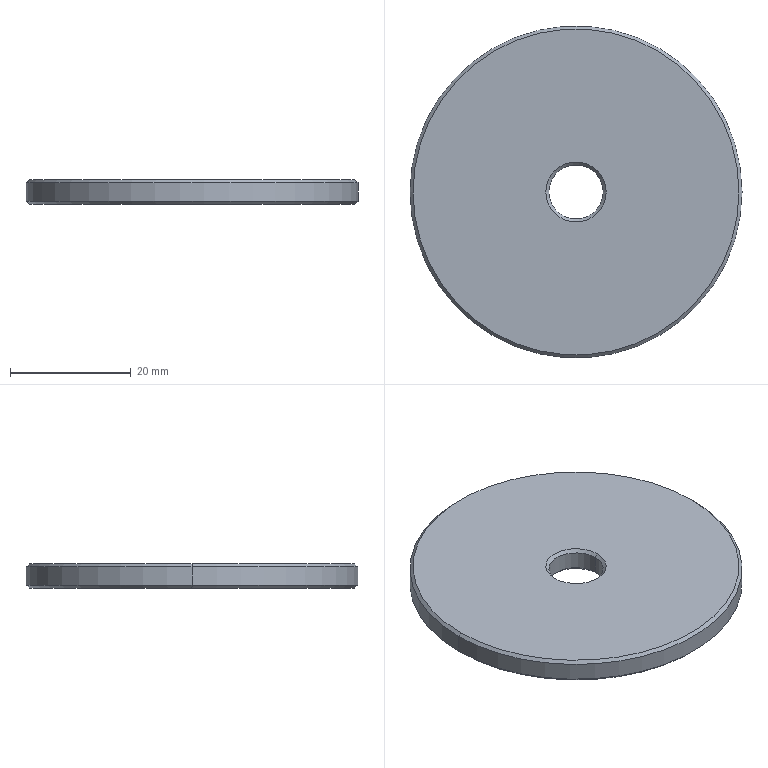Part | SolidWorks | features BaseBody 1 | 1 solid | 14 faces | box 55 x 55 x 4 mm | volume 9199 mm3 | cone 8 | cylinder 4 | plane 2 | commonest cylinder face diameters 9 x2 55 x2
STEP:
#1=CARTESIAN_POINT('',(27.,0.,4.));
#2=VERTEX_POINT('',#1);
#3=CARTESIAN_POINT('',(-27.,0.,4.));
#4=VERTEX_POINT('',#3);
#5=CARTESIAN_POINT('',(0.,0.,4.));
#6=DIRECTION('',(0.,0.,1.));
#7=DIRECTION('',(1.,0.,0.));
#8=AXIS2_PLACEMENT_3D('',#5,#6,#7);
#9=CIRCLE('',#8,27.);
#10=EDGE_CURVE('',#2,#4,#9,.T.);
#11=ORIENTED_EDGE('',*,*,#10,.F.);
#12=CARTESIAN_POINT('',(27.5,0.,3.5));
#13=VERTEX_POINT('',#12);
#14=CARTESIAN_POINT('',(27.,0.,4.));
#15=DIRECTION('',(0.7071,0.,-0.7071));
#16=VECTOR('',#15,1000.);
#17=LINE('',#14,#16);
#18=EDGE_CURVE('',#2,#13,#17,.T.);
#19=ORIENTED_EDGE('',*,*,#18,.T.);
#20=CARTESIAN_POINT('',(-27.5,0.,3.5));
#21=VERTEX_POINT('',#20);
#22=CARTESIAN_POINT('',(0.,0.,3.5));
#23=DIRECTION('',(0.,0.,-1.));
#24=DIRECTION('',(1.,0.,0.));
#25=AXIS2_PLACEMENT_3D('',#22,#23,#24);
#26=CIRCLE('',#25,27.5);
#27=EDGE_CURVE('',#21,#13,#26,.T.);
#28=ORIENTED_EDGE('',*,*,#27,.F.);
#29=CARTESIAN_POINT('',(-27.,0.,4.));
#30=DIRECTION('',(-0.7071,0.,-0.7071));
#31=VECTOR('',#30,1000.);
#32=LINE('',#29,#31);
#33=EDGE_CURVE('',#4,#21,#32,.T.);
#34=ORIENTED_EDGE('',*,*,#33,.F.);
#35=EDGE_LOOP('',(#11,#19,#28,#34));
#36=FACE_OUTER_BOUND('',#35,.T.);
#37=CARTESIAN_POINT('',(0.,0.,4.));
#38=DIRECTION('',(0.,0.,-1.));
#39=DIRECTION('',(-1.,0.,0.));
#40=AXIS2_PLACEMENT_3D('',#37,#38,#39);
#41=CONICAL_SURFACE('',#40,27.,0.7854);
#42=ADVANCED_FACE('',(#36),#41,.T.);
#43=CARTESIAN_POINT('',(-27.,0.,0.));
#44=VERTEX_POINT('',#43);
#45=CARTESIAN_POINT('',(27.,0.,0.));
#46=VERTEX_POINT('',#45);
#47=CARTESIAN_POINT('',(0.,0.,0.));
#48=DIRECTION('',(0.,0.,-1.));
#49=DIRECTION('',(1.,0.,0.));
#50=AXIS2_PLACEMENT_3D('',#47,#48,#49);
#51=CIRCLE('',#50,27.);
#52=EDGE_CURVE('',#44,#46,#51,.T.);
#53=ORIENTED_EDGE('',*,*,#52,.F.);
#54=CARTESIAN_POINT('',(-27.5,0.,0.5));
#55=VERTEX_POINT('',#54);
#56=CARTESIAN_POINT('',(-27.5,0.,0.5));
#57=DIRECTION('',(-0.7071,0.,0.7071));
#58=VECTOR('',#57,1000.);
#59=LINE('',#56,#58);
#60=EDGE_CURVE('',#44,#55,#59,.T.);
#61=ORIENTED_EDGE('',*,*,#60,.T.);
#62=CARTESIAN_POINT('',(27.5,0.,0.5));
#63=VERTEX_POINT('',#62);
#64=CARTESIAN_POINT('',(0.,0.,0.5));
#65=DIRECTION('',(0.,0.,1.));
#66=DIRECTION('',(1.,0.,0.));
#67=AXIS2_PLACEMENT_3D('',#64,#65,#66);
#68=CIRCLE('',#67,27.5);
#69=EDGE_CURVE('',#63,#55,#68,.T.);
#70=ORIENTED_EDGE('',*,*,#69,.F.);
#71=CARTESIAN_POINT('',(27.5,0.,0.5));
#72=DIRECTION('',(0.7071,0.,0.7071));
#73=VECTOR('',#72,1000.);
#74=LINE('',#71,#73);
#75=EDGE_CURVE('',#46,#63,#74,.T.);
#76=ORIENTED_EDGE('',*,*,#75,.F.);
#77=EDGE_LOOP('',(#53,#61,#70,#76));
#78=FACE_OUTER_BOUND('',#77,.T.);
#79=CARTESIAN_POINT('',(0.,0.,0.5));
#80=DIRECTION('',(0.,0.,1.));
#81=DIRECTION('',(1.,0.,0.));
#82=AXIS2_PLACEMENT_3D('',#79,#80,#81);
#83=CONICAL_SURFACE('',#82,27.5,0.7854);
#84=ADVANCED_FACE('',(#78),#83,.T.);
#85=CARTESIAN_POINT('',(4.5,0.,0.5));
#86=VERTEX_POINT('',#85);
#87=CARTESIAN_POINT('',(-4.5,0.,0.5));
#88=VERTEX_POINT('',#87);
#89=CARTESIAN_POINT('',(0.,0.,0.5));
#90=DIRECTION('',(0.,0.,-1.));
#91=DIRECTION('',(1.,0.,0.));
#92=AXIS2_PLACEMENT_3D('',#89,#90,#91);
#93=CIRCLE('',#92,4.5);
#94=EDGE_CURVE('',#86,#88,#93,.T.);
#95=ORIENTED_EDGE('',*,*,#94,.F.);
#96=CARTESIAN_POINT('',(5.,0.,0.));
#97=VERTEX_POINT('',#96);
#98=CARTESIAN_POINT('',(5.,0.,0.));
#99=DIRECTION('',(0.7071,0.,-0.7071));
#100=VECTOR('',#99,1000.);
#101=LINE('',#98,#100);
#102=EDGE_CURVE('',#86,#97,#101,.T.);
#103=ORIENTED_EDGE('',*,*,#102,.T.);
#104=CARTESIAN_POINT('',(-5.,0.,0.));
#105=VERTEX_POINT('',#104);
#106=CARTESIAN_POINT('',(0.,0.,0.));
#107=DIRECTION('',(0.,0.,1.));
#108=DIRECTION('',(1.,0.,0.));
#109=AXIS2_PLACEMENT_3D('',#106,#107,#108);
#110=CIRCLE('',#109,5.);
#111=EDGE_CURVE('',#105,#97,#110,.T.);
#112=ORIENTED_EDGE('',*,*,#111,.F.);
#113=CARTESIAN_POINT('',(-5.,0.,0.));
#114=DIRECTION('',(-0.7071,0.,-0.7071));
#115=VECTOR('',#114,1000.);
#116=LINE('',#113,#115);
#117=EDGE_CURVE('',#88,#105,#116,.T.);
#118=ORIENTED_EDGE('',*,*,#117,.F.);
#119=EDGE_LOOP('',(#95,#103,#112,#118));
#120=FACE_OUTER_BOUND('',#119,.T.);
#121=CARTESIAN_POINT('',(0.,0.,0.));
#122=DIRECTION('',(0.,0.,-1.));
#123=DIRECTION('',(-1.,0.,0.));
#124=AXIS2_PLACEMENT_3D('',#121,#122,#123);
#125=CONICAL_SURFACE('',#124,5.,0.7854);
#126=ADVANCED_FACE('',(#120),#125,.F.);
#127=CARTESIAN_POINT('',(-4.5,0.,3.5));
#128=VERTEX_POINT('',#127);
#129=CARTESIAN_POINT('',(4.5,0.,3.5));
#130=VERTEX_POINT('',#129);
#131=CARTESIAN_POINT('',(0.,0.,3.5));
#132=DIRECTION('',(0.,0.,1.));
#133=DIRECTION('',(1.,0.,0.));
#134=AXIS2_PLACEMENT_3D('',#131,#132,#133);
#135=CIRCLE('',#134,4.5);
#136=EDGE_CURVE('',#128,#130,#135,.T.);
#137=ORIENTED_EDGE('',*,*,#136,.F.);
#138=CARTESIAN_POINT('',(-5.,0.,4.));
#139=VERTEX_POINT('',#138);
#140=CARTESIAN_POINT('',(-4.5,0.,3.5));
#141=DIRECTION('',(-0.7071,0.,0.7071));
#142=VECTOR('',#141,1000.);
#143=LINE('',#140,#142);
#144=EDGE_CURVE('',#128,#139,#143,.T.);
#145=ORIENTED_EDGE('',*,*,#144,.T.);
#146=CARTESIAN_POINT('',(5.,0.,4.));
#147=VERTEX_POINT('',#146);
#148=CARTESIAN_POINT('',(0.,0.,4.));
#149=DIRECTION('',(0.,0.,-1.));
#150=DIRECTION('',(1.,0.,0.));
#151=AXIS2_PLACEMENT_3D('',#148,#149,#150);
#152=CIRCLE('',#151,5.);
#153=EDGE_CURVE('',#147,#139,#152,.T.);
#154=ORIENTED_EDGE('',*,*,#153,.F.);
#155=CARTESIAN_POINT('',(4.5,0.,3.5));
#156=DIRECTION('',(0.7071,0.,0.7071));
#157=VECTOR('',#156,1000.);
#158=LINE('',#155,#157);
#159=EDGE_CURVE('',#130,#147,#158,.T.);
#160=ORIENTED_EDGE('',*,*,#159,.F.);
#161=EDGE_LOOP('',(#137,#145,#154,#160));
#162=FACE_OUTER_BOUND('',#161,.T.);
#163=CARTESIAN_POINT('',(0.,0.,3.5));
#164=DIRECTION('',(0.,0.,1.));
#165=DIRECTION('',(1.,0.,0.));
#166=AXIS2_PLACEMENT_3D('',#163,#164,#165);
#167=CONICAL_SURFACE('',#166,4.5,0.7854);
#168=ADVANCED_FACE('',(#162),#167,.F.);
#169=ORIENTED_EDGE('',*,*,#136,.T.);
#170=CARTESIAN_POINT('',(4.5,0.,4.));
#171=DIRECTION('',(0.,0.,-1.));
#172=VECTOR('',#171,1000.);
#173=LINE('',#170,#172);
#174=EDGE_CURVE('',#130,#86,#173,.T.);
#175=ORIENTED_EDGE('',*,*,#174,.T.);
#176=ORIENTED_EDGE('',*,*,#94,.T.);
#177=CARTESIAN_POINT('',(-4.5,0.,4.));
#178=DIRECTION('',(0.,0.,-1.));
#179=VECTOR('',#178,1000.);
#180=LINE('',#177,#179);
#181=EDGE_CURVE('',#128,#88,#180,.T.);
#182=ORIENTED_EDGE('',*,*,#181,.F.);
#183=EDGE_LOOP('',(#169,#175,#176,#182));
#184=FACE_OUTER_BOUND('',#183,.T.);
#185=CARTESIAN_POINT('',(0.,0.,4.));
#186=DIRECTION('',(0.,0.,-1.));
#187=DIRECTION('',(-1.,0.,0.));
#188=AXIS2_PLACEMENT_3D('',#185,#186,#187);
#189=CYLINDRICAL_SURFACE('',#188,4.5);
#190=ADVANCED_FACE('',(#184),#189,.F.);
#191=ORIENTED_EDGE('',*,*,#27,.T.);
#192=CARTESIAN_POINT('',(27.5,0.,4.));
#193=DIRECTION('',(0.,0.,-1.));
#194=VECTOR('',#193,1000.);
#195=LINE('',#192,#194);
#196=EDGE_CURVE('',#13,#63,#195,.T.);
#197=ORIENTED_EDGE('',*,*,#196,.T.);
#198=ORIENTED_EDGE('',*,*,#69,.T.);
#199=CARTESIAN_POINT('',(-27.5,0.,4.));
#200=DIRECTION('',(0.,0.,-1.));
#201=VECTOR('',#200,1000.);
#202=LINE('',#199,#201);
#203=EDGE_CURVE('',#21,#55,#202,.T.);
#204=ORIENTED_EDGE('',*,*,#203,.F.);
#205=EDGE_LOOP('',(#191,#197,#198,#204));
#206=FACE_OUTER_BOUND('',#205,.T.);
#207=CARTESIAN_POINT('',(0.,0.,4.));
#208=DIRECTION('',(0.,0.,-1.));
#209=DIRECTION('',(-1.,0.,0.));
#210=AXIS2_PLACEMENT_3D('',#207,#208,#209);
#211=CYLINDRICAL_SURFACE('',#210,27.5);
#212=ADVANCED_FACE('',(#206),#211,.T.);
#213=ORIENTED_EDGE('',*,*,#153,.T.);
#214=CARTESIAN_POINT('',(0.,0.,4.));
#215=DIRECTION('',(0.,0.,-1.));
#216=DIRECTION('',(1.,0.,0.));
#217=AXIS2_PLACEMENT_3D('',#214,#215,#216);
#218=CIRCLE('',#217,5.);
#219=EDGE_CURVE('',#139,#147,#218,.T.);
#220=ORIENTED_EDGE('',*,*,#219,.T.);
#221=EDGE_LOOP('',(#213,#220));
#222=FACE_BOUND('',#221,.T.);
#223=CARTESIAN_POINT('',(0.,0.,4.));
#224=DIRECTION('',(0.,0.,1.));
#225=DIRECTION('',(1.,0.,0.));
#226=AXIS2_PLACEMENT_3D('',#223,#224,#225);
#227=CIRCLE('',#226,27.);
#228=EDGE_CURVE('',#4,#2,#227,.T.);
#229=ORIENTED_EDGE('',*,*,#228,.T.);
#230=ORIENTED_EDGE('',*,*,#10,.T.);
#231=EDGE_LOOP('',(#229,#230));
#232=FACE_OUTER_BOUND('',#231,.T.);
#233=CARTESIAN_POINT('',(0.,0.,4.));
#234=DIRECTION('',(0.,0.,1.));
#235=DIRECTION('',(1.,0.,0.));
#236=AXIS2_PLACEMENT_3D('',#233,#234,#235);
#237=PLANE('',#236);
#238=ADVANCED_FACE('',(#222,#232),#237,.T.);
#239=ORIENTED_EDGE('',*,*,#111,.T.);
#240=CARTESIAN_POINT('',(0.,0.,0.));
#241=DIRECTION('',(0.,0.,1.));
#242=DIRECTION('',(1.,0.,0.));
#243=AXIS2_PLACEMENT_3D('',#240,#241,#242);
#244=CIRCLE('',#243,5.);
#245=EDGE_CURVE('',#97,#105,#244,.T.);
#246=ORIENTED_EDGE('',*,*,#245,.T.);
#247=EDGE_LOOP('',(#239,#246));
#248=FACE_BOUND('',#247,.T.);
#249=CARTESIAN_POINT('',(0.,0.,0.));
#250=DIRECTION('',(0.,0.,-1.));
#251=DIRECTION('',(1.,0.,0.));
#252=AXIS2_PLACEMENT_3D('',#249,#250,#251);
#253=CIRCLE('',#252,27.);
#254=EDGE_CURVE('',#46,#44,#253,.T.);
#255=ORIENTED_EDGE('',*,*,#254,.T.);
#256=ORIENTED_EDGE('',*,*,#52,.T.);
#257=EDGE_LOOP('',(#255,#256));
#258=FACE_OUTER_BOUND('',#257,.T.);
#259=CARTESIAN_POINT('',(0.,0.,0.));
#260=DIRECTION('',(0.,0.,1.));
#261=DIRECTION('',(1.,0.,0.));
#262=AXIS2_PLACEMENT_3D('',#259,#260,#261);
#263=PLANE('',#262);
#264=ADVANCED_FACE('',(#248,#258),#263,.F.);
#265=ORIENTED_EDGE('',*,*,#196,.F.);
#266=CARTESIAN_POINT('',(0.,0.,3.5));
#267=DIRECTION('',(0.,0.,-1.));
#268=DIRECTION('',(1.,0.,0.));
#269=AXIS2_PLACEMENT_3D('',#266,#267,#268);
#270=CIRCLE('',#269,27.5);
#271=EDGE_CURVE('',#13,#21,#270,.T.);
#272=ORIENTED_EDGE('',*,*,#271,.T.);
#273=ORIENTED_EDGE('',*,*,#203,.T.);
#274=CARTESIAN_POINT('',(0.,0.,0.5));
#275=DIRECTION('',(0.,0.,1.));
#276=DIRECTION('',(1.,0.,0.));
#277=AXIS2_PLACEMENT_3D('',#274,#275,#276);
#278=CIRCLE('',#277,27.5);
#279=EDGE_CURVE('',#55,#63,#278,.T.);
#280=ORIENTED_EDGE('',*,*,#279,.T.);
#281=EDGE_LOOP('',(#265,#272,#273,#280));
#282=FACE_OUTER_BOUND('',#281,.T.);
#283=CARTESIAN_POINT('',(0.,0.,4.));
#284=DIRECTION('',(0.,0.,-1.));
#285=DIRECTION('',(-1.,0.,0.));
#286=AXIS2_PLACEMENT_3D('',#283,#284,#285);
#287=CYLINDRICAL_SURFACE('',#286,27.5);
#288=ADVANCED_FACE('',(#282),#287,.T.);
#289=ORIENTED_EDGE('',*,*,#174,.F.);
#290=CARTESIAN_POINT('',(0.,0.,3.5));
#291=DIRECTION('',(0.,0.,1.));
#292=DIRECTION('',(1.,0.,0.));
#293=AXIS2_PLACEMENT_3D('',#290,#291,#292);
#294=CIRCLE('',#293,4.5);
#295=EDGE_CURVE('',#130,#128,#294,.T.);
#296=ORIENTED_EDGE('',*,*,#295,.T.);
#297=ORIENTED_EDGE('',*,*,#181,.T.);
#298=CARTESIAN_POINT('',(0.,0.,0.5));
#299=DIRECTION('',(0.,0.,-1.));
#300=DIRECTION('',(1.,0.,0.));
#301=AXIS2_PLACEMENT_3D('',#298,#299,#300);
#302=CIRCLE('',#301,4.5);
#303=EDGE_CURVE('',#88,#86,#302,.T.);
#304=ORIENTED_EDGE('',*,*,#303,.T.);
#305=EDGE_LOOP('',(#289,#296,#297,#304));
#306=FACE_OUTER_BOUND('',#305,.T.);
#307=CARTESIAN_POINT('',(0.,0.,4.));
#308=DIRECTION('',(0.,0.,-1.));
#309=DIRECTION('',(-1.,0.,0.));
#310=AXIS2_PLACEMENT_3D('',#307,#308,#309);
#311=CYLINDRICAL_SURFACE('',#310,4.5);
#312=ADVANCED_FACE('',(#306),#311,.F.);
#313=ORIENTED_EDGE('',*,*,#144,.F.);
#314=ORIENTED_EDGE('',*,*,#295,.F.);
#315=ORIENTED_EDGE('',*,*,#159,.T.);
#316=ORIENTED_EDGE('',*,*,#219,.F.);
#317=EDGE_LOOP('',(#313,#314,#315,#316));
#318=FACE_OUTER_BOUND('',#317,.T.);
#319=CARTESIAN_POINT('',(0.,0.,3.5));
#320=DIRECTION('',(0.,0.,1.));
#321=DIRECTION('',(1.,0.,0.));
#322=AXIS2_PLACEMENT_3D('',#319,#320,#321);
#323=CONICAL_SURFACE('',#322,4.5,0.7854);
#324=ADVANCED_FACE('',(#318),#323,.F.);
#325=ORIENTED_EDGE('',*,*,#102,.F.);
#326=ORIENTED_EDGE('',*,*,#303,.F.);
#327=ORIENTED_EDGE('',*,*,#117,.T.);
#328=ORIENTED_EDGE('',*,*,#245,.F.);
#329=EDGE_LOOP('',(#325,#326,#327,#328));
#330=FACE_OUTER_BOUND('',#329,.T.);
#331=CARTESIAN_POINT('',(0.,0.,0.));
#332=DIRECTION('',(0.,0.,-1.));
#333=DIRECTION('',(-1.,0.,0.));
#334=AXIS2_PLACEMENT_3D('',#331,#332,#333);
#335=CONICAL_SURFACE('',#334,5.,0.7854);
#336=ADVANCED_FACE('',(#330),#335,.F.);
#337=ORIENTED_EDGE('',*,*,#60,.F.);
#338=ORIENTED_EDGE('',*,*,#254,.F.);
#339=ORIENTED_EDGE('',*,*,#75,.T.);
#340=ORIENTED_EDGE('',*,*,#279,.F.);
#341=EDGE_LOOP('',(#337,#338,#339,#340));
#342=FACE_OUTER_BOUND('',#341,.T.);
#343=CARTESIAN_POINT('',(0.,0.,0.5));
#344=DIRECTION('',(0.,0.,1.));
#345=DIRECTION('',(1.,0.,0.));
#346=AXIS2_PLACEMENT_3D('',#343,#344,#345);
#347=CONICAL_SURFACE('',#346,27.5,0.7854);
#348=ADVANCED_FACE('',(#342),#347,.T.);
#349=ORIENTED_EDGE('',*,*,#18,.F.);
#350=ORIENTED_EDGE('',*,*,#228,.F.);
#351=ORIENTED_EDGE('',*,*,#33,.T.);
#352=ORIENTED_EDGE('',*,*,#271,.F.);
#353=EDGE_LOOP('',(#349,#350,#351,#352));
#354=FACE_OUTER_BOUND('',#353,.T.);
#355=CARTESIAN_POINT('',(0.,0.,4.));
#356=DIRECTION('',(0.,0.,-1.));
#357=DIRECTION('',(-1.,0.,0.));
#358=AXIS2_PLACEMENT_3D('',#355,#356,#357);
#359=CONICAL_SURFACE('',#358,27.,0.7854);
#360=ADVANCED_FACE('',(#354),#359,.T.);
#361=CLOSED_SHELL('',(#42,#84,#126,#168,#190,#212,#238,#264,#288,#312,#324,#336,#348,#360));
#362=MANIFOLD_SOLID_BREP('',#361);
#363=CARTESIAN_POINT('',(0.,0.,0.));
#364=DIRECTION('',(0.,0.,1.));
#365=DIRECTION('',(1.,0.,0.));
#366=AXIS2_PLACEMENT_3D('',#363,#364,#365);
#367=(LENGTH_UNIT()NAMED_UNIT(*)SI_UNIT(.MILLI.,.METRE.));
#368=UNCERTAINTY_MEASURE_WITH_UNIT(LENGTH_MEASURE(0.00001),#367,'','');
#369=(NAMED_UNIT(*)PLANE_ANGLE_UNIT()SI_UNIT($,.RADIAN.));
#370=(NAMED_UNIT(*)SI_UNIT($,.STERADIAN.)SOLID_ANGLE_UNIT());
#371=(GEOMETRIC_REPRESENTATION_CONTEXT(3)GLOBAL_UNCERTAINTY_ASSIGNED_CONTEXT((#368))GLOBAL_UNIT_ASSIGNED_CONTEXT((#367,#369,#370))REPRESENTATION_CONTEXT('',''));
#372=ADVANCED_BREP_SHAPE_REPRESENTATION('',(#362,#366),#371);